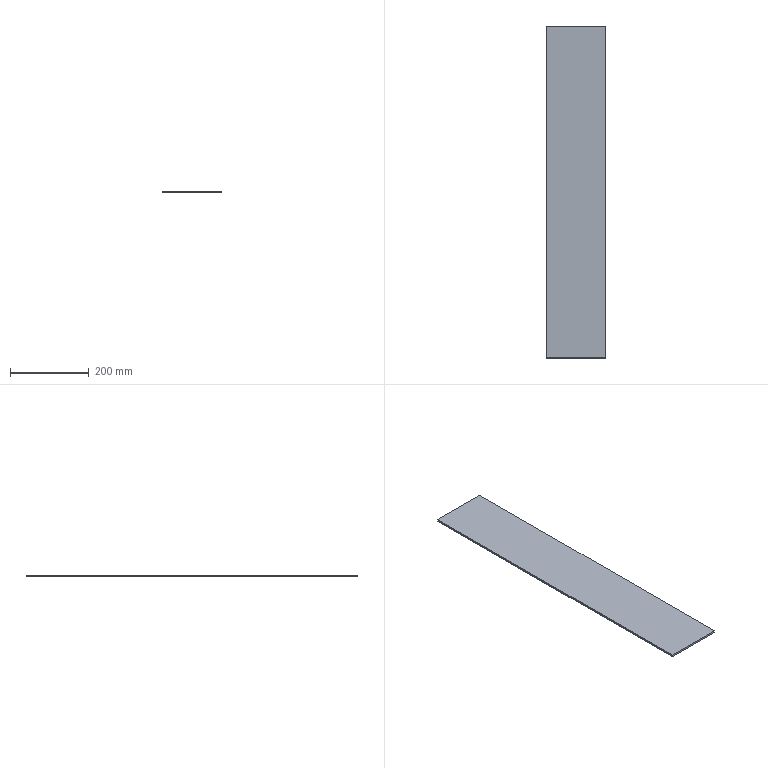Part | SolidWorks | features Extrusion 1, HoleWzd 1 | 1 solid | 6 faces | box 151 x 842 x 5 mm | volume 635710 mm3 | plane 6
STEP:
#1=CARTESIAN_POINT('',(75.5,-421.,0.));
#2=VERTEX_POINT('',#1);
#3=CARTESIAN_POINT('',(75.5,421.,0.));
#4=VERTEX_POINT('',#3);
#5=CARTESIAN_POINT('',(75.5,421.,0.));
#6=DIRECTION('',(0.,1.,0.));
#7=VECTOR('',#6,1000.);
#8=LINE('',#5,#7);
#9=EDGE_CURVE('',#2,#4,#8,.T.);
#10=ORIENTED_EDGE('',*,*,#9,.T.);
#11=CARTESIAN_POINT('',(75.5,421.,5.));
#12=VERTEX_POINT('',#11);
#13=CARTESIAN_POINT('',(75.5,421.,5.));
#14=DIRECTION('',(0.,0.,-1.));
#15=VECTOR('',#14,1000.);
#16=LINE('',#13,#15);
#17=EDGE_CURVE('',#12,#4,#16,.T.);
#18=ORIENTED_EDGE('',*,*,#17,.F.);
#19=CARTESIAN_POINT('',(75.5,-421.,5.));
#20=VERTEX_POINT('',#19);
#21=CARTESIAN_POINT('',(75.5,421.,5.));
#22=DIRECTION('',(0.,1.,0.));
#23=VECTOR('',#22,1000.);
#24=LINE('',#21,#23);
#25=EDGE_CURVE('',#20,#12,#24,.T.);
#26=ORIENTED_EDGE('',*,*,#25,.F.);
#27=CARTESIAN_POINT('',(75.5,-421.,5.));
#28=DIRECTION('',(0.,0.,-1.));
#29=VECTOR('',#28,1000.);
#30=LINE('',#27,#29);
#31=EDGE_CURVE('',#20,#2,#30,.T.);
#32=ORIENTED_EDGE('',*,*,#31,.T.);
#33=EDGE_LOOP('',(#10,#18,#26,#32));
#34=FACE_OUTER_BOUND('',#33,.T.);
#35=CARTESIAN_POINT('',(75.5,421.,5.));
#36=DIRECTION('',(-1.,0.,0.));
#37=DIRECTION('',(0.,-1.,0.));
#38=AXIS2_PLACEMENT_3D('',#35,#36,#37);
#39=PLANE('',#38);
#40=ADVANCED_FACE('',(#34),#39,.F.);
#41=CARTESIAN_POINT('',(-75.5,421.,0.));
#42=VERTEX_POINT('',#41);
#43=CARTESIAN_POINT('',(-75.5,421.,0.));
#44=DIRECTION('',(-1.,0.,0.));
#45=VECTOR('',#44,1000.);
#46=LINE('',#43,#45);
#47=EDGE_CURVE('',#4,#42,#46,.T.);
#48=ORIENTED_EDGE('',*,*,#47,.T.);
#49=CARTESIAN_POINT('',(-75.5,421.,5.));
#50=VERTEX_POINT('',#49);
#51=CARTESIAN_POINT('',(-75.5,421.,5.));
#52=DIRECTION('',(0.,0.,-1.));
#53=VECTOR('',#52,1000.);
#54=LINE('',#51,#53);
#55=EDGE_CURVE('',#50,#42,#54,.T.);
#56=ORIENTED_EDGE('',*,*,#55,.F.);
#57=CARTESIAN_POINT('',(-75.5,421.,5.));
#58=DIRECTION('',(-1.,0.,0.));
#59=VECTOR('',#58,1000.);
#60=LINE('',#57,#59);
#61=EDGE_CURVE('',#12,#50,#60,.T.);
#62=ORIENTED_EDGE('',*,*,#61,.F.);
#63=ORIENTED_EDGE('',*,*,#17,.T.);
#64=EDGE_LOOP('',(#48,#56,#62,#63));
#65=FACE_OUTER_BOUND('',#64,.T.);
#66=CARTESIAN_POINT('',(-75.5,421.,5.));
#67=DIRECTION('',(0.,-1.,0.));
#68=DIRECTION('',(0.,0.,-1.));
#69=AXIS2_PLACEMENT_3D('',#66,#67,#68);
#70=PLANE('',#69);
#71=ADVANCED_FACE('',(#65),#70,.F.);
#72=CARTESIAN_POINT('',(-75.5,-421.,0.));
#73=VERTEX_POINT('',#72);
#74=CARTESIAN_POINT('',(-75.5,421.,0.));
#75=DIRECTION('',(0.,-1.,0.));
#76=VECTOR('',#75,1000.);
#77=LINE('',#74,#76);
#78=EDGE_CURVE('',#42,#73,#77,.T.);
#79=ORIENTED_EDGE('',*,*,#78,.T.);
#80=CARTESIAN_POINT('',(-75.5,-421.,5.));
#81=VERTEX_POINT('',#80);
#82=CARTESIAN_POINT('',(-75.5,-421.,5.));
#83=DIRECTION('',(0.,0.,-1.));
#84=VECTOR('',#83,1000.);
#85=LINE('',#82,#84);
#86=EDGE_CURVE('',#81,#73,#85,.T.);
#87=ORIENTED_EDGE('',*,*,#86,.F.);
#88=CARTESIAN_POINT('',(-75.5,421.,5.));
#89=DIRECTION('',(0.,-1.,0.));
#90=VECTOR('',#89,1000.);
#91=LINE('',#88,#90);
#92=EDGE_CURVE('',#50,#81,#91,.T.);
#93=ORIENTED_EDGE('',*,*,#92,.F.);
#94=ORIENTED_EDGE('',*,*,#55,.T.);
#95=EDGE_LOOP('',(#79,#87,#93,#94));
#96=FACE_OUTER_BOUND('',#95,.T.);
#97=CARTESIAN_POINT('',(-75.5,421.,5.));
#98=DIRECTION('',(1.,0.,0.));
#99=DIRECTION('',(0.,1.,0.));
#100=AXIS2_PLACEMENT_3D('',#97,#98,#99);
#101=PLANE('',#100);
#102=ADVANCED_FACE('',(#96),#101,.F.);
#103=CARTESIAN_POINT('',(-75.5,-421.,0.));
#104=DIRECTION('',(1.,0.,0.));
#105=VECTOR('',#104,1000.);
#106=LINE('',#103,#105);
#107=EDGE_CURVE('',#73,#2,#106,.T.);
#108=ORIENTED_EDGE('',*,*,#107,.T.);
#109=ORIENTED_EDGE('',*,*,#31,.F.);
#110=CARTESIAN_POINT('',(-75.5,-421.,5.));
#111=DIRECTION('',(1.,0.,0.));
#112=VECTOR('',#111,1000.);
#113=LINE('',#110,#112);
#114=EDGE_CURVE('',#81,#20,#113,.T.);
#115=ORIENTED_EDGE('',*,*,#114,.F.);
#116=ORIENTED_EDGE('',*,*,#86,.T.);
#117=EDGE_LOOP('',(#108,#109,#115,#116));
#118=FACE_OUTER_BOUND('',#117,.T.);
#119=CARTESIAN_POINT('',(-75.5,-421.,5.));
#120=DIRECTION('',(0.,1.,0.));
#121=DIRECTION('',(0.,0.,1.));
#122=AXIS2_PLACEMENT_3D('',#119,#120,#121);
#123=PLANE('',#122);
#124=ADVANCED_FACE('',(#118),#123,.F.);
#125=ORIENTED_EDGE('',*,*,#25,.T.);
#126=ORIENTED_EDGE('',*,*,#61,.T.);
#127=ORIENTED_EDGE('',*,*,#92,.T.);
#128=ORIENTED_EDGE('',*,*,#114,.T.);
#129=EDGE_LOOP('',(#125,#126,#127,#128));
#130=FACE_OUTER_BOUND('',#129,.T.);
#131=CARTESIAN_POINT('',(0.,0.,5.));
#132=DIRECTION('',(0.,0.,1.));
#133=DIRECTION('',(1.,0.,0.));
#134=AXIS2_PLACEMENT_3D('',#131,#132,#133);
#135=PLANE('',#134);
#136=ADVANCED_FACE('',(#130),#135,.T.);
#137=ORIENTED_EDGE('',*,*,#9,.F.);
#138=ORIENTED_EDGE('',*,*,#107,.F.);
#139=ORIENTED_EDGE('',*,*,#78,.F.);
#140=ORIENTED_EDGE('',*,*,#47,.F.);
#141=EDGE_LOOP('',(#137,#138,#139,#140));
#142=FACE_OUTER_BOUND('',#141,.T.);
#143=CARTESIAN_POINT('',(0.,0.,0.));
#144=DIRECTION('',(0.,0.,1.));
#145=DIRECTION('',(1.,0.,0.));
#146=AXIS2_PLACEMENT_3D('',#143,#144,#145);
#147=PLANE('',#146);
#148=ADVANCED_FACE('',(#142),#147,.F.);
#149=CLOSED_SHELL('',(#40,#71,#102,#124,#136,#148));
#150=MANIFOLD_SOLID_BREP('',#149);
#151=CARTESIAN_POINT('',(0.,0.,0.));
#152=DIRECTION('',(0.,0.,1.));
#153=DIRECTION('',(1.,0.,0.));
#154=AXIS2_PLACEMENT_3D('',#151,#152,#153);
#155=(LENGTH_UNIT()NAMED_UNIT(*)SI_UNIT(.MILLI.,.METRE.));
#156=UNCERTAINTY_MEASURE_WITH_UNIT(LENGTH_MEASURE(0.00001),#155,'','');
#157=(NAMED_UNIT(*)PLANE_ANGLE_UNIT()SI_UNIT($,.RADIAN.));
#158=(NAMED_UNIT(*)SI_UNIT($,.STERADIAN.)SOLID_ANGLE_UNIT());
#159=(GEOMETRIC_REPRESENTATION_CONTEXT(3)GLOBAL_UNCERTAINTY_ASSIGNED_CONTEXT((#156))GLOBAL_UNIT_ASSIGNED_CONTEXT((#155,#157,#158))REPRESENTATION_CONTEXT('',''));
#160=ADVANCED_BREP_SHAPE_REPRESENTATION('',(#150,#154),#159);